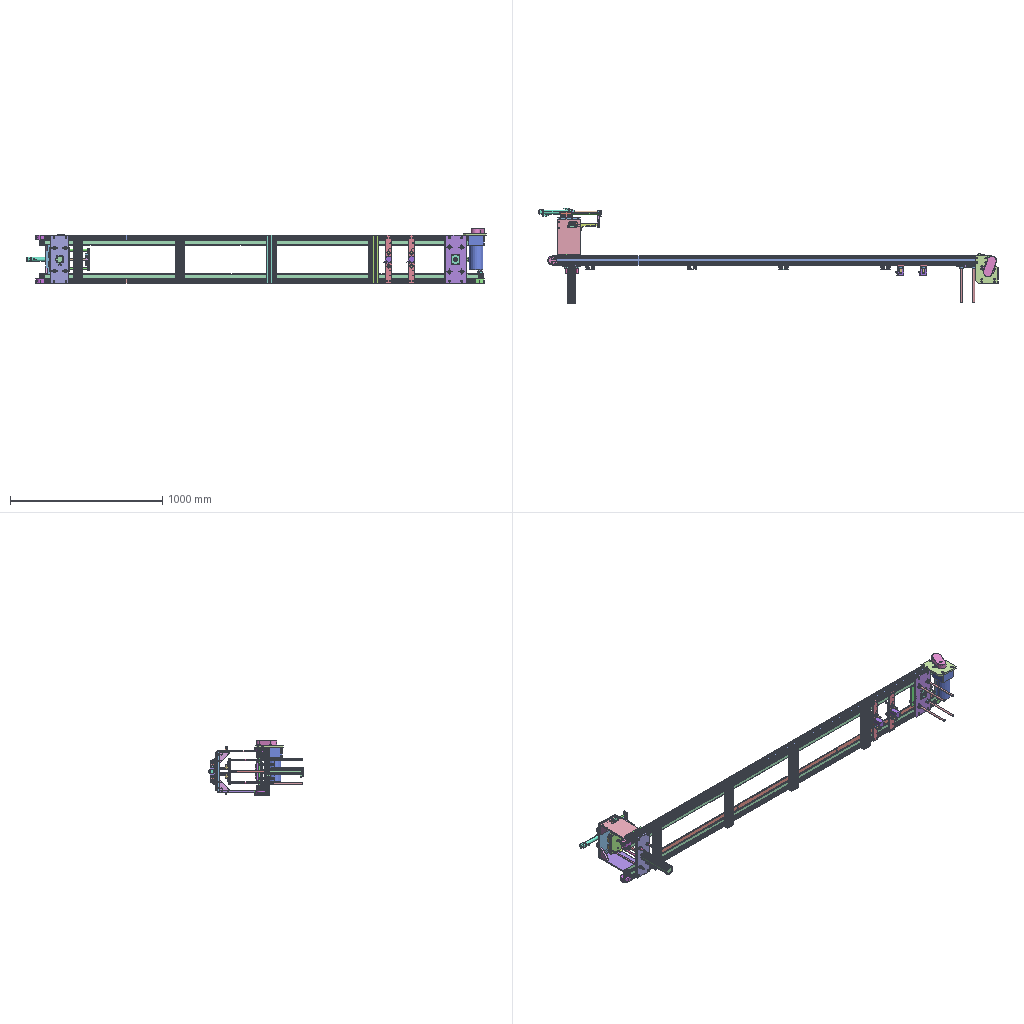Assembly | STEP file | 75 different items | 137 placed | box 3024 x 631 x 361 mm
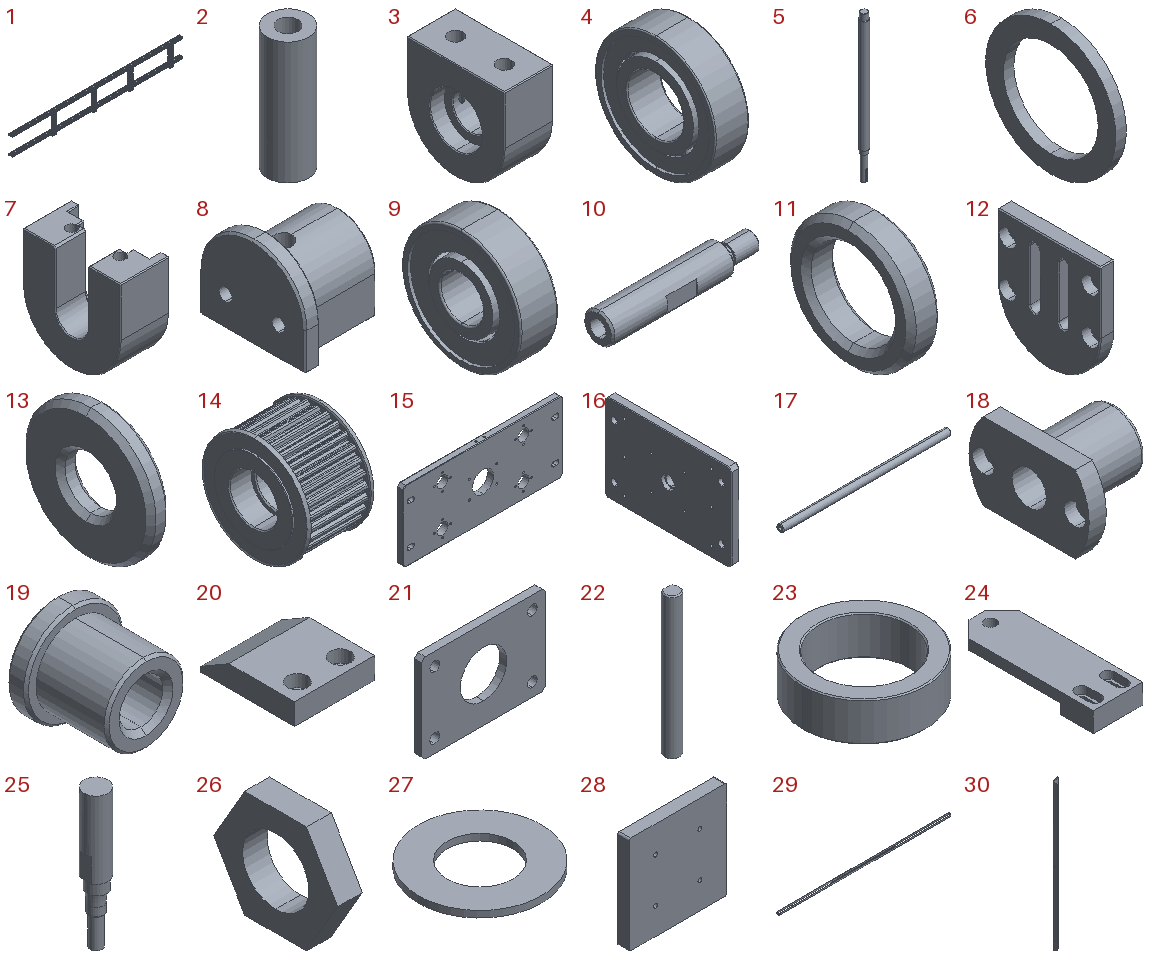Parts list (item | name | quantity | parent item | size | volume):
1 | Reflow conveyor bracket_Default | x1 | - | 2830 x 90 x 316 mm | 3898026 mm3
2 | CB-M-15-17 Threaded bushing_Default | x8 | - | 10 x 10 x 30 mm | 1767 mm3
3 | - | x2 | - | 30 x 60 x 60 mm | 72459 mm3
4 | GB/T276-94 Deep groove ball bearing 6002-2Z | x2 | - | 9 x 32 x 32 mm | 3545 mm3
5 | - | x1 | - | 18 x 18 x 335 mm | 73475 mm3
6 | - | x2 | - | 2 x 25 x 25 mm | 461.437 mm3
7 | - | x2 | in Driven wheel assembly_Default | 30 x 60 x 60 mm | 50936 mm3
8 | - | x2 | in Driven wheel assembly_Default | 23 x 28 x 24 mm | 8364 mm3
9 | GB/T276-94 Deep groove ball bearing 608-2Z | x4 | in Driven wheel assembly_Default | 7 x 22 x 22 mm | 1460 mm3
10 | - | x2 | in Driven wheel assembly_Default | 40.5 x 8 x 8 mm | 1575 mm3
11 | - | x2 | in Driven wheel assembly_Default | 3 x 12 x 12 mm | 168.916 mm3
12 | - | x2 | in Driven wheel assembly_Default | 7 x 50 x 55 mm | 14443 mm3
13 | - | x2 | in Driven wheel assembly_Default | 2 x 13 x 13 mm | 208.696 mm3
14 | - | x2 | in Driven wheel assembly_Default | 32 x 49 x 49 mm | 40684 mm3
15 | - | x1 | in Frame_Default | 316 x 12 x 140 mm | 486609 mm3
16 | - | x1 | in Frame_Default | 12 x 190 x 130 mm | 287114 mm3
17 | - | x4 | in Frame_Default | 280 x 12 x 12 mm | 31385 mm3
18 | LHFC12_LHFC12 | x4 | in Frame_Default | 30 x 42 x 27 mm | 10763 mm3
19 | - | x1 | in Frame_Default | 19.8 x 18 x 19.8 mm | 2819 mm3
20 | - | x2 | in Frame_Default | 30 x 35 x 8 mm | 6950 mm3
21 | - | x1 | in Frame_Default | 70 x 4 x 50 mm | 11431 mm3
22 | - | x2 | in Frame_Default | 14 x 12 x 130 mm | 17958 mm3
23 | - | x1 | in Frame_Default | 22 x 22 x 7 mm | 1249 mm3
24 | - | x1 | in Frame_Default | 30 x 85 x 12 mm | 16342 mm3
25 | E2E_X2D1_N_BASE | x1 | in Proximity sensor E2E_X2D1_N | 8 x 8 x 47 mm | 1680 mm3
26 | E2E_X2D1_N_NUT | x2 | in Proximity sensor E2E_X2D1_N | 3 x 15.011 x 13 mm | 288.278 mm3
27 | E2E_X2D1_N_WASHER | x1 | in Proximity sensor E2E_X2D1_N | 15 x 15 x 0.8 mm | 101.159 mm3
28 | Urethane pad block_Default | x1 | in Frame_Default | 110 x 13 x 110 mm | 155824 mm3
29 | Belt 1-11^Default | x2 | - | 2922 x 49 x 25 mm | 294683 mm3
30 | - | x6 | - | 35 x 30 x 929.978 mm | 113908 mm3
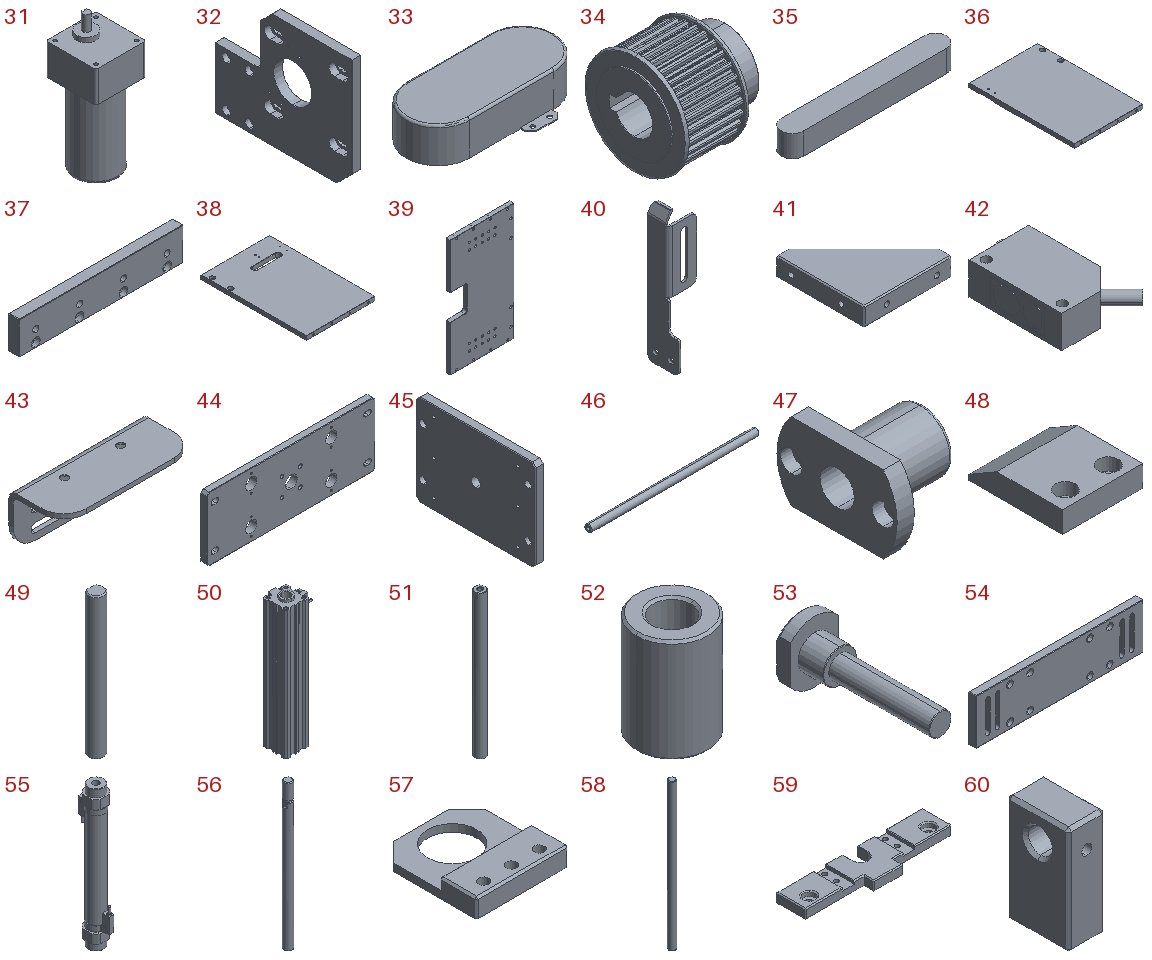31 | Motor 90W_Default | x1 | - | 104 x 104 x 269 mm | 1739193 mm3
32 | - | x1 | - | 12 x 180 x 150 mm | 230112 mm3
33 | - | x1 | - | 140 x 80 x 33 mm | 18882 mm3
34 | - | x2 | - | 44 x 49 x 49 mm | 49129 mm3
35 | - | x2 | - | 45 x 6 x 6 mm | 1574 mm3
36 | PN_0001-002 Blanking support plate1_Default | x1 | in PN_0001 Blanking support plate assembly_Default | 150 x 230 x 9 mm | 307149 mm3
37 | PN_0001-003 Blanking support plate2_Default | x2 | in PN_0001 Blanking support plate assembly_Default | 150 x 10 x 30 mm | 41531 mm3
38 | PN_0001-001 Blanking support plate_Default | x1 | in PN_0001 Blanking support plate assembly_Default | 150 x 230 x 9 mm | 300493 mm3
39 | PN_0001-004 Blanking support plate3_Default | x1 | in PN_0001 Blanking support plate assembly_Default | 150 x 10 x 274 mm | 378327 mm3
40 | PN_0001-008 Alignment plate_Default | x1 | in PN_0001 Blanking support plate assembly_Default | 27 x 30 x 130 mm | 7946 mm3
41 | PN_0001-006 Reinforcing rib_Default | x2 | in PN_0001 Blanking support plate assembly_Default | 70 x 70 x 15 mm | 45416 mm3
42 | Photoelectric sensor E3Z_LS61 | x1 | in PN_0001 Blanking support plate assembly_Default | 24.985 x 38.085 x 10.8 mm | 6465 mm3
43 | PN_0002-17 Sensor fixing plate_Default | x1 | in PN_0001 Blanking support plate assembly_Default | 60 x 25 x 24 mm | 4566 mm3
44 | PN_0001-17 Blanking linear bearing mounting plate_Default | x1 | in Frame-2 | 316 x 12 x 120 mm | 422737 mm3
45 | PN_0001-18 Blanking lift plate_Default | x1 | in Frame-2 | 12 x 170 x 130 mm | 257545 mm3
46 | - | x4 | in Frame-2 | 280 x 12 x 12 mm | 31385 mm3
47 | LHFC12-2_LHFC12 | x4 | in Frame-2 | 30 x 42 x 27 mm | 10763 mm3
48 | - | x2 | in Frame-2 | 30 x 35 x 8 mm | 6950 mm3
49 | - | x2 | in Frame-2 | 14 x 12 x 130 mm | 17958 mm3
50 | A_CDQ2A32-200DC-F7NV(0)_Default | x1 | in CDQ2A-200_Default | 63.2 x 49.5 x 249.5 mm | 394520 mm3
51 | A_CDQ2A32-200DC-F7NV(0) - Main body_Default | x1 | in Frame-2 | 16 x 16 x 218 mm | 43283 mm3
52 | PN_0001-19 Cylinder extension shaft_Default | x1 | in Frame-2 | 16 x 16 x 23 mm | 3300 mm3
53 | PN_0001-20 Cylinder connecting spacer screw_Default | x1 | in Frame-2 | 17 x 50.1 x 22 mm | 4480 mm3
54 | PN_0001-09 Pusher fixing plate_Default | x1 | in Pusher assembly_Default | 256 x 12 x 70 mm | 193349 mm3
55 | A_CDM2B25-150-C76(0)_Default | x1 | in CDM-25-150_Default | 30 x 52.6 x 238 mm | 131860 mm3
56 | A_CDM2B25-150-C76(1)_Default | x1 | in CDM-25-150_Default | 10 x 10 x 183 mm | 14238 mm3
57 | PN_0001-10 Pusher cylinder fixing plate_Default | x1 | in Pusher assembly_Default | 50 x 55 x 10 mm | 13598 mm3
58 | PN_0001-11 12 Locking rod_Default | x2 | in Pusher assembly_Default | 12 x 12 x 270 mm | 30254 mm3
59 | PN_0001-13 Rotating support plate_Default | x1 | in Pusher assembly_Default | 150 x 40 x 10 mm | 40974 mm3
60 | PN_0001-14 Pusher rotating shaft fixing plate_Default | x2 | in Pusher assembly_Default | 12 x 20 x 35 mm | 7342 mm3
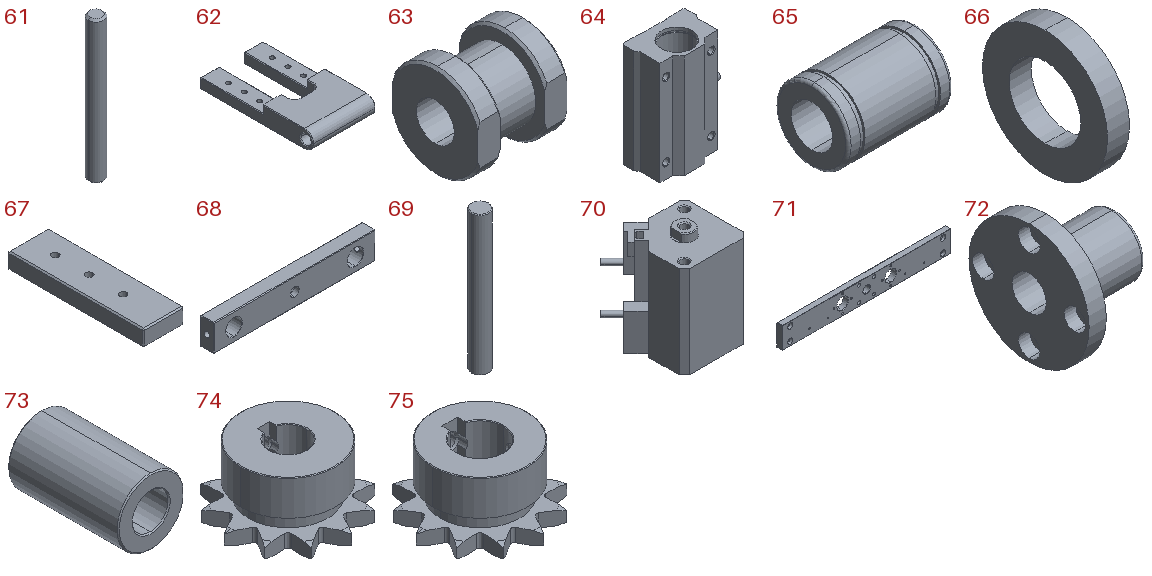61 | PN_0001-15 10 Rotating shaft_Default | x1 | in Pusher assembly_Default | 8 x 8 x 74 mm | 3697 mm3
62 | PN_0001-16 Pusher plate_Default | x1 | in Pusher assembly_Default | 50 x 90 x 14 mm | 32757 mm3
63 | PN_0001-12 Pusher cylinder connection block_Default | x1 | in Pusher assembly_Default | 20 x 19 x 21 mm | 3951 mm3
64 | LHBBW12body_Default | x2 | in LHBBW12_LHBBW12, Pusher assembly_Default | 49 x 28 x 70 mm | 46534 mm3
65 | LMU12_Default | x2 | in LHBBW12_LHBBW12 | 30 x 21 x 21 mm | 6896 mm3
66 | LHBBW12collar3_Default | x1 | in LHBBW12_LHBBW12 | 3.7 x 21 x 21 mm | 863.074 mm3
67 | PN_0001-21 Anti-collision block_Default | x2 | in Pusher assembly_Default | 15 x 50 x 6 mm | 4377 mm3
68 | PN_0002-07 Connection plate_Default | x2 | in Universal test stopper 12_Default | 120 x 10 x 20 mm | 20677 mm3
69 | PN_0002-08 Test alignment rod_Default | x4 | in Universal test stopper 12_Default | 12 x 12 x 95 mm | 10735 mm3
70 | A_CDQ2A25-25D-F7NV012_Default | x2 | in Universal test stopper 12_Default | 52.598 x 52.598 x 62.5 mm | 85379 mm3
71 | PN_0002-06 Stopper cylinder seat_Default | x2 | in Universal test stopper 12_Default | 316 x 10 x 40 mm | 112914 mm3
72 | LHFR122_Default | x4 | in Universal test stopper 12_Default | 30 x 42 x 42 mm | 12352 mm3
73 | PN_0002-09 Cylinder extension rod_Default | x2 | in Universal test stopper 12_Default | 12 x 20 x 12 mm | 1596 mm3
74 | SP35B12_N_12_SP35B12-N-12 | x1 | - | 41 x 41 x 20 mm | 11740 mm3
75 | SP35B12_N_15_SP35B12-N-15 | x1 | - | 41 x 41 x 20 mm | 10343 mm3
Placements (level | parent | child | x y z in mm | rotation matrix by rows):
1 | subassembly 2 | Reflow conveyor bracket_Default | -0.0 -0.0 -0.0 | -1 0 0 0 1 0 0 0 -1
1 | subassembly 2 | CB-M-15-17 Threaded bushing_Default | 1385.0 15.0 -143.0 | 0 0 1 0 1 0 -1 0 0
1 | subassembly 2 | CB-M-15-17 Threaded bushing_Default | 1385.0 -15.0 -143.0 | 0 0 1 0.9242 -0.3818 0 0.3818 0.9242 0
1 | subassembly 2 | CB-M-15-17 Threaded bushing_Default | -1415.0 -15.0 143.0 | 0 0 1 0.007845 1 0 -1 0.007845 0
1 | subassembly 2 | CB-M-15-17 Threaded bushing_Default | -1415.0 15.0 143.0 | 0 0 1 0 1 0 -1 0 0
1 | subassembly 2 | CB-M-15-17 Threaded bushing_Default | -1415.0 15.0 -143.0 | 0 0 1 0 1 0 -1 0 0
1 | subassembly 2 | CB-M-15-17 Threaded bushing_Default | -1415.0 -15.0 -143.0 | 0 0 1 0 1 0 -1 0 0
1 | subassembly 2 | CB-M-15-17 Threaded bushing_Default | 1385.0 -15.0 143.0 | 0 0 1 0 1 0 -1 0 0
1 | subassembly 2 | CB-M-15-17 Threaded bushing_Default | 1385.0 15.0 143.0 | 0 0 1 0 1 0 -1 0 0
1 | subassembly 2 | subassembly 3 | 1430.0 0.0 -128.0 | 0 0 -1 0 -1 0 -1 0 0
1 | subassembly 2 | subassembly 3 | 1430.0 -0.0 128.0 | 0 0 -1 0 1 0 1 0 0
1 | subassembly 2 | GB/T276-94 Deep groove ball bearing 6002-2Z | 1445.0 0.0 132.5 | 0 -0.9907 0.1358 0 -0.1358 -0.9907 1 0 -0
1 | subassembly 2 | GB/T276-94 Deep groove ball bearing 6002-2Z | 1445.0 0.0 -132.5 | 0 0 -1 0 1 0 1 0 0
1 | subassembly 2 | subassembly 4 | 1445.0 0.0 -142.0 | -0.2677 0.9635 0 0.9635 0.2677 0 0 0 -1
1 | subassembly 2 | subassembly 5 | 1445.0 0.0 126.0 | 0 0 -1 0 1 0 1 0 0
1 | subassembly 2 | subassembly 5 | 1445.0 0.0 -128.0 | 0 0 -1 0 1 0 1 0 0
1 | subassembly 2 | Driven wheel assembly_Default | -1430.0 -0.0 128.0 | 0 0 1 0 -1 0 1 0 0
2 | Driven wheel assembly_Default | subassembly 6 | -0.0 -0.0 -0.0 | 1 0 0 0 1 0 0 0 1
2 | Driven wheel assembly_Default | subassembly 7 | 23.0 0.0 15.0 | -1 0 0 0 1 0 0 0 -1
2 | Driven wheel assembly_Default | GB/T276-94 Deep groove ball bearing 608-2Z | -27.5 -0.0 2.73 | 1 0 0 0 -0.000286 -1 0 1 -0.000286
2 | Driven wheel assembly_Default | subassembly 8 | -32.5 0.0 2.73 | 1 0 0 0 -1 0 0 0 -1
2 | Driven wheel assembly_Default | GB/T276-94 Deep groove ball bearing 608-2Z | -6.5 -0.0 2.73 | -1 0 0 0 -0.9992 0.03909 0 0.03909 0.9992
2 | Driven wheel assembly_Default | subassembly 9 | -0.0 0.0 2.73 | -1 0 0 0 0.1471 -0.9891 0 -0.9891 -0.1471
2 | Driven wheel assembly_Default | subassembly 10 | 30.0 -0.0 15.0 | -1 0 0 0 -1 0 0 0 1
2 | Driven wheel assembly_Default | subassembly 11 | -33.0 -0.0 2.73 | 1 0 0 0 0.9757 0.2192 0 -0.2192 0.9757
2 | Driven wheel assembly_Default | subassembly 12 | -34.0 -0.0 2.73 | 1 0 0 0 1 0 0 0 1
1 | subassembly 2 | Driven wheel assembly_Default | -1430.0 0.0 -128.0 | 0 0 1 0 1 0 -1 0 -0
2 | Driven wheel assembly_Default | subassembly 6 | -0.0 -0.0 -0.0 | 1 0 0 0 1 0 0 0 1
2 | Driven wheel assembly_Default | subassembly 7 | 23.0 0.0 15.0 | -1 0 0 0 1 0 0 0 -1
2 | Driven wheel assembly_Default | GB/T276-94 Deep groove ball bearing 608-2Z | -27.5 -0.0 2.73 | 1 0 0 0 -0.000286 -1 0 1 -0.000286
2 | Driven wheel assembly_Default | subassembly 8 | -32.5 0.0 2.73 | 1 0 0 0 -1 0 0 0 -1
2 | Driven wheel assembly_Default | GB/T276-94 Deep groove ball bearing 608-2Z | -6.5 -0.0 2.73 | -1 0 0 0 -0.9992 0.03909 0 0.03909 0.9992
2 | Driven wheel assembly_Default | subassembly 9 | -0.0 0.0 2.73 | -1 0 0 0 0.1471 -0.9891 0 -0.9891 -0.1471
2 | Driven wheel assembly_Default | subassembly 10 | 30.0 -0.0 15.0 | -1 0 0 0 -1 0 0 0 1
2 | Driven wheel assembly_Default | subassembly 11 | -33.0 -0.0 2.73 | 1 0 0 0 0.9757 0.2192 0 -0.2192 0.9757
2 | Driven wheel assembly_Default | subassembly 12 | -34.0 -0.0 2.73 | 1 0 0 0 1 0 0 0 1
1 | subassembly 2 | Frame_Default | 1288.35 13.745 -33.168 | 0 0 -1 0 1 0 1 0 0
2 | Frame_Default | subassembly 13 | 33.168 -55.745 3.35 | 1 0 0 0 1 0 0 0 1
2 | Frame_Default | subassembly 14 | 33.168 -1.645 3.35 | 0 1 0 -1 0 0 0 0 1
2 | Frame_Default | subassembly 15 | 113.168 -13.645 -36.65 | 0 0.9719 0.2354 -1 0 0 0 -0.2354 0.9719
2 | Frame_Default | subassembly 15 | 113.168 -13.645 43.35 | 0 0.6574 -0.7536 -1 0 0 0 0.7536 0.6574
2 | Frame_Default | LHFC12_LHFC12 | 113.168 -37.745 -36.65 | 0 1 0 -1 0 0 0 0 1
2 | Frame_Default | LHFC12_LHFC12 | 113.168 -37.745 43.35 | 0 1 0 -1 0 0 0 0 1
2 | Frame_Default | subassembly 16 | 33.168 -20.745 3.35 | 1 0 0 0 1 0 0 0 1
2 | Frame_Default | subassembly 17 | 3.168 -7.645 -65.65 | -1 0 0 0 1 0 0 0 -1
2 | Frame_Default | subassembly 18 | 33.168 -55.745 3.35 | 1 0 0 0 1 0 0 0 1
2 | Frame_Default | LHFC12_LHFC12 | -46.832 -37.745 -36.65 | 0 1 0 -1 0 0 0 0 1
2 | Frame_Default | LHFC12_LHFC12 | -46.832 -37.745 43.35 | 0 1 0 -1 0 0 0 0 1
2 | Frame_Default | subassembly 15 | -46.832 -13.645 43.35 | 0 0.6574 -0.7536 -1 0 0 0 0.7536 0.6574
2 | Frame_Default | subassembly 15 | -46.832 -13.645 -36.65 | 0 0.6574 -0.7536 -1 0 0 0 0.7536 0.6574
2 | Frame_Default | subassembly 17 | 63.168 -7.645 -65.65 | -1 0 0 0 1 0 0 0 -1
2 | Frame_Default | subassembly 19 | -31.832 3.355 68.35 | 1 0 0 0 -1 0 0 0 -1
2 | Frame_Default | subassembly 19 | 98.168 3.355 68.35 | 1 0 0 0 -1 0 0 0 -1
2 | Frame_Default | subassembly 20 | 33.168 -17.145 3.35 | 1 0 0 0 0 1 0 -1 -0
2 | Frame_Default | subassembly 21 | 33.168 -49.745 -72.65 | -1 0 0 0 1 0 0 0 -1
2 | Frame_Default | Proximity sensor E2E_X2D1_N | 33.168 21.255 -61.65 | 1 0 0 0 1 0 0 0 1
3 | Proximity sensor E2E_X2D1_N | E2E_X2D1_N_BASE | -0.0 -0.0 0.0 | 1 0 0 0 1 0 0 0 1
3 | Proximity sensor E2E_X2D1_N | E2E_X2D1_N_NUT | -0.0 -0.0 -11.0 | 0 0 -1 0 1 0 1 0 0
3 | Proximity sensor E2E_X2D1_N | E2E_X2D1_N_NUT | -0.0 -0.0 -16.8 | 0 0 -1 0 1 0 1 0 0
3 | Proximity sensor E2E_X2D1_N | E2E_X2D1_N_WASHER | -0.0 -0.0 -13.0 | 1 0 0 0 1 0 0 0 1
2 | Frame_Default | Urethane pad block_Default | 33.168 -1.645 3.35 | 1 0 0 0 1 0 0 0 1
1 | subassembly 2 | Belt 1-11^Default | 1445.73 -0.0 -97.5 | -1 0 0 0 -1 0 0 0 1
1 | subassembly 2 | Belt 1-11^Default | 1445.73 0.0 122.5 | -1 0 0 0 -1 0 0 0 1
1 | subassembly 2 | subassembly 22 | 993.236 15.0 -110.5 | 0 0 -1 0 1 0 1 0 0
1 | subassembly 2 | subassembly 22 | 920.0 15.0 110.5 | 0 0 1 0 1 0 -1 0 -0
1 | subassembly 2 | Motor 90W_Default | 1420.0 -90.0 93.0 | 1 0 0 0 1 0 0 0 1
1 | subassembly 2 | subassembly 23 | 1410.0 -60.0 170.0 | 0 0 1 0 1 0 -1 0 -0
1 | subassembly 2 | subassembly 24 | 1445.349 -2.359 170.0 | -0.342 0.9397 0 -0.9397 -0.342 0 0 0 1
1 | subassembly 2 | subassembly 22 | 0.0 15.0 110.5 | 0 0 1 0 1 0 -1 0 -0
1 | subassembly 2 | subassembly 22 | -920.0 15.0 110.5 | 0 0 1 0 1 0 -1 0 -0
1 | subassembly 2 | subassembly 22 | 73.236 15.0 -110.5 | 0 0 -1 0 1 0 1 0 0
1 | subassembly 2 | subassembly 22 | -846.764 15.0 -110.5 | 0 0 -1 0 1 0 1 0 0
1 | subassembly 2 | subassembly 25 | 1445.0 -0.0 126.0 | 0 0.9635 0.2677 0 0.2677 -0.9635 -1 0 0
1 | subassembly 2 | subassembly 25 | 1445.0 -0.0 -126.0 | 0 0.9635 -0.2677 0 0.2677 0.9635 1 0 -0
1 | subassembly 2 | subassembly 26 | 1453.19 2.275 102.5 | 0 -0.2677 -0.9635 0 0.9635 -0.2677 1 0 0
1 | subassembly 2 | subassembly 26 | 1453.19 2.275 -103.5 | 0 -0.2677 -0.9635 0 0.9635 -0.2677 1 0 0
1 | subassembly 2 | PN_0001 Blanking support plate assembly_Default | -1335.0 155.0 -128.0 | -1 0 0 0 1 0 0 0 -1
2 | PN_0001 Blanking support plate assembly_Default | PN_0001-002 Blanking support plate1_Default | -0.0 -0.0 -0.0 | 1 0 0 0 1 0 0 0 1
2 | PN_0001 Blanking support plate assembly_Default | PN_0001-003 Blanking support plate2_Default | -0.0 -125.0 15.0 | 1 0 0 0 1 0 0 0 1
2 | PN_0001 Blanking support plate assembly_Default | PN_0001-001 Blanking support plate_Default | -0.0 -0.0 -256.0 | -1 0 0 0 1 0 0 0 -1
2 | PN_0001 Blanking support plate assembly_Default | PN_0001-003 Blanking support plate2_Default | 0.0 -125.0 -271.0 | -1 0 0 0 1 0 0 0 -1
2 | PN_0001 Blanking support plate assembly_Default | PN_0001-004 Blanking support plate3_Default | -0.0 115.0 -128.0 | 1 0 0 0 1 0 0 0 1
2 | PN_0001 Blanking support plate assembly_Default | PN_0001-008 Alignment plate_Default | -70.0 75.0 1.8 | 0 0 -1 0 1 0 1 0 -0
2 | PN_0001 Blanking support plate assembly_Default | PN_0001-006 Reinforcing rib_Default | 60.0 80.0 -35.0 | 0 0 1 -1 0 0 0 -1 -0
2 | PN_0001 Blanking support plate assembly_Default | PN_0001-006 Reinforcing rib_Default | 75.0 80.0 -221.0 | 0 0 -1 -1 0 0 0 1 0
2 | PN_0001 Blanking support plate assembly_Default | Photoelectric sensor E3Z_LS61 | -36.179 69.0 -273.0 | 0 1 0 0 0 -1 -1 0 0
2 | PN_0001 Blanking support plate assembly_Default | PN_0002-17 Sensor fixing plate_Default | -23.479 74.4 -277.5 | 1 0 0 0 0 -1 0 1 0
1 | subassembly 2 | Frame-2 | -1320.35 13.745 33.168 | 0 0 1 0 1 0 -1 0 0
2 | Frame-2 | PN_0001-17 Blanking linear bearing mounting plate_Default | 33.168 -55.745 3.35 | 1 0 0 0 1 0 0 0 1
2 | Frame-2 | PN_0001-18 Blanking lift plate_Default | 33.168 193.255 3.35 | 0 1 0 -1 0 0 0 0 1
2 | Frame-2 | subassembly 27 | 108.168 181.255 -31.65 | 0 0.8804 0.4742 -1 0 0 0 -0.4742 0.8804
2 | Frame-2 | subassembly 27 | 108.168 181.255 38.35 | 0 0.6574 -0.7536 -1 0 0 0 0.7536 0.6574
2 | Frame-2 | LHFC12-2_LHFC12 | 108.168 -37.745 -31.65 | 0 0 1 -1 0 0 0 -1 -0
2 | Frame-2 | LHFC12-2_LHFC12 | 108.168 -37.745 38.35 | 0 0 1 -1 0 0 0 -1 0
2 | Frame-2 | subassembly 28 | 3.168 187.255 -65.65 | -1 0 0 0 1 0 0 0 -1
2 | Frame-2 | LHFC12-2_LHFC12 | -41.832 -37.745 -31.65 | 0 0 -1 -1 0 0 0 1 -0
2 | Frame-2 | LHFC12-2_LHFC12 | -41.832 -37.745 38.35 | 0 0 -1 -1 0 0 0 1 -0
2 | Frame-2 | subassembly 27 | -41.832 181.255 38.35 | 0 0.897 0.442 -1 0 0 0 -0.442 0.897
2 | Frame-2 | subassembly 27 | -41.832 181.255 -31.65 | 0 0.6574 -0.7536 -1 0 0 0 0.7536 0.6574
2 | Frame-2 | subassembly 28 | 63.168 187.255 -65.65 | -1 0 0 0 1 0 0 0 -1
2 | Frame-2 | subassembly 29 | -26.832 198.255 68.35 | 1 0 0 0 -1 0 0 0 -1
2 | Frame-2 | subassembly 29 | 93.168 198.255 68.35 | 1 0 0 0 -1 0 0 0 -1
2 | Frame-2 | CDQ2A-200_Default | 33.168 -55.745 3.35 | 1 0 0 0 0 1 0 -1 0
3 | CDQ2A-200_Default | A_CDQ2A32-200DC-F7NV(0)_Default | -0.0 -0.0 -0.0 | 1 0 0 0 1 0 0 0 1
2 | Frame-2 | A_CDQ2A32-200DC-F7NV(0) - Main body_Default | 33.168 144.255 3.35 | 0.9055 0.4242 0 0 0 1 0.4242 -0.9055 0
2 | Frame-2 | PN_0001-19 Cylinder extension shaft_Default | 33.168 184.255 3.35 | 1 0 0 0 0 -1 0 1 -0
2 | Frame-2 | PN_0001-20 Cylinder connecting spacer screw_Default | 33.168 148.155 3.35 | 1 0 0 0 1 0 0 0 1
1 | subassembly 2 | Pusher assembly_Default | -1355.377 280.0 -0.0 | 0 0 -1 0 1 0 1 0 0
2 | Pusher assembly_Default | PN_0001-09 Pusher fixing plate_Default | -0.0 -0.0 -0.0 | 1 0 0 0 1 0 0 0 1
2 | Pusher assembly_Default | CDM-25-150_Default | 0.0 38.0 -54.0 | -0.9991 -0.04323 0 -0.04323 0.9991 0 0 0 -1
3 | CDM-25-150_Default | A_CDM2B25-150-C76(0)_Default | 0.0 -0.0 -0.0 | 1 0 0 0 1 0 0 0 1
3 | CDM-25-150_Default | A_CDM2B25-150-C76(1)_Default | -0.0 0.0 150.0 | 1 0 0 0 1 0 0 0 1
2 | Pusher assembly_Default | PN_0001-10 Pusher cylinder fixing plate_Default | 0.0 27.5 -45.0 | 1 0 0 0 1 0 0 0 1
2 | Pusher assembly_Default | PN_0001-11 12 Locking rod_Default | 61.0 27.0 -226.0 | 0.9706 -0.2405 0 0.2405 0.9706 0 0 0 1
2 | Pusher assembly_Default | PN_0001-11 12 Locking rod_Default | -61.0 28.0 -226.0 | -0.7326 0.6807 0 -0.6807 -0.7326 0 0 0 1
2 | Pusher assembly_Default | PN_0001-13 Rotating support plate_Default | 0.0 28.0 -231.0 | 1 0 0 0 1 0 0 0 1
2 | Pusher assembly_Default | PN_0001-14 Pusher rotating shaft fixing plate_Default | 31.0 30.5 -204.0 | -1 0 0 0 0 -1 0 -1 0
2 | Pusher assembly_Default | PN_0001-14 Pusher rotating shaft fixing plate_Default | -31.0 30.5 -204.0 | -1 0 0 0 0 -1 0 -1 0
2 | Pusher assembly_Default | PN_0001-15 10 Rotating shaft_Default | -36.962 21.5 -214.0 | 0 0 -1 0 1 0 1 0 -0
2 | Pusher assembly_Default | PN_0001-16 Pusher plate_Default | 0.0 -17.292 -205.925 | 1 0 0 0 -0.9996 -0.02763 0 0.02763 -0.9996
2 | Pusher assembly_Default | PN_0001-12 Pusher cylinder connection block_Default | 0.0 38.0 -236.0 | 0 0.9977 0.06756 0 -0.06756 0.9977 1 0 -0
2 | Pusher assembly_Default | LHBBW12_LHBBW12 | -61.0 27.0 -0.0 | -1 0 0 0 -1 0 0 0 1
3 | LHBBW12_LHBBW12 | LHBBW12body_Default | -0.0 -0.0 -0.0 | 1 0 0 0 1 0 0 0 1
3 | LHBBW12_LHBBW12 | LMU12_Default | -0.0 -1.0 1.85 | 0 0 -1 0 1 0 1 0 -0
3 | LHBBW12_LHBBW12 | LMU12_Default | -0.0 -1.0 -31.85 | 0 0 -1 0 1 0 1 0 -0
3 | LHBBW12_LHBBW12 | LHBBW12collar3_Default | -0.0 -1.0 0.0 | 0 0 -1 0 1 0 1 0 -0
2 | Pusher assembly_Default | LHBBW12body_Default | 61.0 27.0 -0.0 | -1 0 0 0 -1 0 0 0 1
2 | Pusher assembly_Default | PN_0001-21 Anti-collision block_Default | 17.5 -37.671 -219.367 | 1 0 0 0 0.9996 0.02763 0 -0.02763 0.9996
2 | Pusher assembly_Default | PN_0001-21 Anti-collision block_Default | -17.5 -37.671 -219.367 | 1 0 0 0 0.9996 0.02763 0 -0.02763 0.9996
1 | subassembly 2 | Universal test stopper 12_Default | 843.25 19.522 -1.088 | 0 0 -1 0 1 0 1 0 0
2 | Universal test stopper 12_Default | PN_0002-07 Connection plate_Default | 1.088 -34.522 -1.75 | 1 0 0 0 1 0 0 0 1
2 | Universal test stopper 12_Default | PN_0002-08 Test alignment rod_Default | 46.088 -7.522 -1.75 | -0.03222 -0.9995 0 0 0 -1 0.9995 -0.03222 -0
2 | Universal test stopper 12_Default | PN_0002-08 Test alignment rod_Default | -43.912 -7.522 -1.75 | -0.1831 -0.9831 0 0 0 -1 0.9831 -0.1831 0
2 | Universal test stopper 12_Default | A_CDQ2A25-25D-F7NV012_Default | 1.088 -59.522 -1.75 | -0.008539 -1 0 0 0 1 -1 0.008539 0
2 | Universal test stopper 12_Default | PN_0002-06 Stopper cylinder seat_Default | 1.088 -59.522 -1.75 | 1 0 0 0 1 0 0 0 1
2 | Universal test stopper 12_Default | LHFR122_Default | 46.088 -43.522 -1.75 | 0 1 0 -1 0 0 0 0 1
2 | Universal test stopper 12_Default | LHFR122_Default | -43.912 -43.522 -1.75 | 0 0 -1 -1 0 0 0 1 0
2 | Universal test stopper 12_Default | PN_0002-09 Cylinder extension rod_Default | 1.088 -54.522 -1.75 | 1 0 0 0 1 0 0 0 1
1 | subassembly 2 | Universal test stopper 12_Default | 993.25 19.522 -1.088 | 0 0 -1 0 1 0 1 0 0
2 | Universal test stopper 12_Default | PN_0002-07 Connection plate_Default | 1.088 -34.522 -1.75 | 1 0 0 0 1 0 0 0 1
2 | Universal test stopper 12_Default | PN_0002-08 Test alignment rod_Default | 46.088 -7.522 -1.75 | -0.03222 -0.9995 0 0 0 -1 0.9995 -0.03222 -0
2 | Universal test stopper 12_Default | PN_0002-08 Test alignment rod_Default | -43.912 -7.522 -1.75 | -0.1831 -0.9831 0 0 0 -1 0.9831 -0.1831 0
2 | Universal test stopper 12_Default | A_CDQ2A25-25D-F7NV012_Default | 1.088 -59.522 -1.75 | -0.008539 -1 0 0 0 1 -1 0.008539 0
2 | Universal test stopper 12_Default | PN_0002-06 Stopper cylinder seat_Default | 1.088 -59.522 -1.75 | 1 0 0 0 1 0 0 0 1
2 | Universal test stopper 12_Default | LHFR122_Default | 46.088 -43.522 -1.75 | 0 1 0 -1 0 0 0 0 1
2 | Universal test stopper 12_Default | LHFR122_Default | -43.912 -43.522 -1.75 | 0 0 -1 -1 0 0 0 1 0
2 | Universal test stopper 12_Default | PN_0002-09 Cylinder extension rod_Default | 1.088 -54.522 -1.75 | 1 0 0 0 1 0 0 0 1
1 | subassembly 2 | SP35B12_N_12_SP35B12-N-12 | 1445.0 0.0 175.0 | 1 0 0 0 1 0 0 0 1
1 | subassembly 2 | SP35B12_N_15_SP35B12-N-15 | 1420.0 -70.0 175.0 | 1 0 0 0 1 0 0 0 1